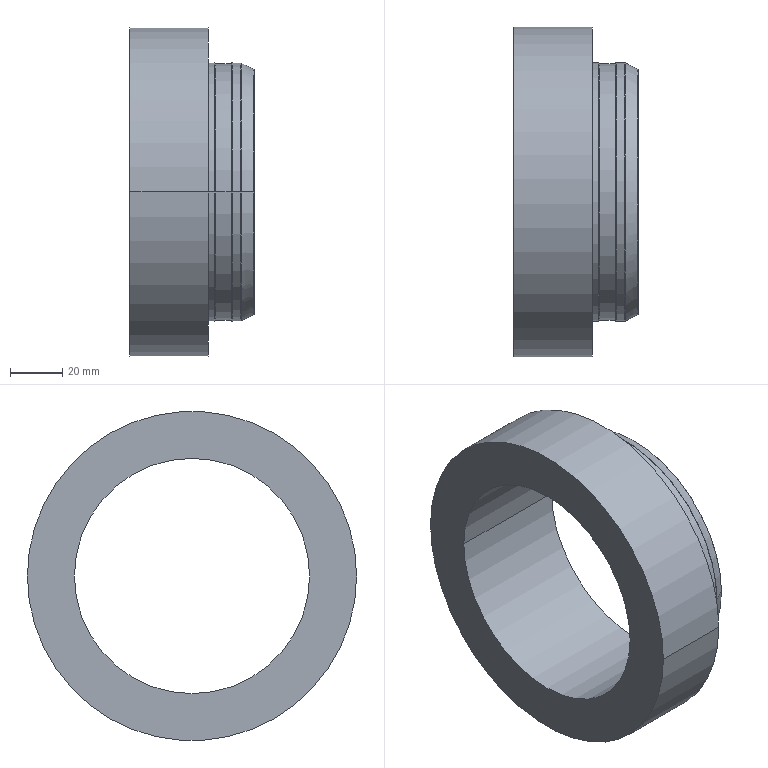Part | SolidWorks | features Revolution 1 | 1 solid | 29 faces | box 47.5 x 126 x 126 mm | volume 203542 mm3 | torus 14 | cylinder 10 | plane 5 | commonest cylinder face diameters 99 x4 90 x2 98 x2 126 x2
STEP:
#1=CARTESIAN_POINT('',(174.371,-47.05,0.));
#2=VERTEX_POINT('',#1);
#3=CARTESIAN_POINT('',(174.371,47.05,0.));
#4=VERTEX_POINT('',#3);
#5=CARTESIAN_POINT('',(174.371,0.,0.));
#6=DIRECTION('',(1.,0.,0.));
#7=DIRECTION('',(0.,1.,0.));
#8=AXIS2_PLACEMENT_3D('',#5,#6,#7);
#9=CIRCLE('',#8,47.05);
#10=EDGE_CURVE('',#2,#4,#9,.T.);
#11=ORIENTED_EDGE('',*,*,#10,.F.);
#12=CARTESIAN_POINT('',(169.544,-49.471,0.));
#13=VERTEX_POINT('',#12);
#14=CARTESIAN_POINT('',(186.323,-76.904,0.));
#15=DIRECTION('',(0.,0.,1.));
#16=DIRECTION('',(0.,-1.,0.));
#17=AXIS2_PLACEMENT_3D('',#14,#15,#16);
#18=CIRCLE('',#17,32.158);
#19=EDGE_CURVE('',#2,#13,#18,.T.);
#20=ORIENTED_EDGE('',*,*,#19,.T.);
#21=CARTESIAN_POINT('',(169.544,49.471,0.));
#22=VERTEX_POINT('',#21);
#23=CARTESIAN_POINT('',(169.544,0.,0.));
#24=DIRECTION('',(1.,0.,0.));
#25=DIRECTION('',(0.,1.,0.));
#26=AXIS2_PLACEMENT_3D('',#23,#24,#25);
#27=CIRCLE('',#26,49.471);
#28=EDGE_CURVE('',#13,#22,#27,.T.);
#29=ORIENTED_EDGE('',*,*,#28,.T.);
#30=CARTESIAN_POINT('',(186.323,76.904,0.));
#31=DIRECTION('',(0.,0.,-1.));
#32=DIRECTION('',(-1.,0.,0.));
#33=AXIS2_PLACEMENT_3D('',#30,#31,#32);
#34=CIRCLE('',#33,32.158);
#35=EDGE_CURVE('',#4,#22,#34,.T.);
#36=ORIENTED_EDGE('',*,*,#35,.F.);
#37=EDGE_LOOP('',(#11,#20,#29,#36));
#38=FACE_OUTER_BOUND('',#37,.T.);
#39=CARTESIAN_POINT('',(186.323,0.,0.));
#40=DIRECTION('',(1.,0.,0.));
#41=DIRECTION('',(0.,1.,0.));
#42=AXIS2_PLACEMENT_3D('',#39,#40,#41);
#43=TOROIDAL_SURFACE('',#42,76.904,32.158);
#44=ADVANCED_FACE('',(#38),#43,.F.);
#45=CARTESIAN_POINT('',(174.371,0.,0.));
#46=DIRECTION('',(1.,0.,0.));
#47=DIRECTION('',(0.,1.,0.));
#48=AXIS2_PLACEMENT_3D('',#45,#46,#47);
#49=CIRCLE('',#48,47.05);
#50=EDGE_CURVE('',#4,#2,#49,.T.);
#51=ORIENTED_EDGE('',*,*,#50,.T.);
#52=CARTESIAN_POINT('',(174.496,-46.864,0.));
#53=VERTEX_POINT('',#52);
#54=CARTESIAN_POINT('',(174.296,-46.864,0.));
#55=DIRECTION('',(0.,0.,1.));
#56=DIRECTION('',(0.,-1.,0.));
#57=AXIS2_PLACEMENT_3D('',#54,#55,#56);
#58=CIRCLE('',#57,0.2);
#59=EDGE_CURVE('',#2,#53,#58,.T.);
#60=ORIENTED_EDGE('',*,*,#59,.T.);
#61=CARTESIAN_POINT('',(174.496,46.864,0.));
#62=VERTEX_POINT('',#61);
#63=CARTESIAN_POINT('',(174.496,0.,0.));
#64=DIRECTION('',(1.,0.,0.));
#65=DIRECTION('',(0.,1.,0.));
#66=AXIS2_PLACEMENT_3D('',#63,#64,#65);
#67=CIRCLE('',#66,46.864);
#68=EDGE_CURVE('',#62,#53,#67,.T.);
#69=ORIENTED_EDGE('',*,*,#68,.F.);
#70=CARTESIAN_POINT('',(174.296,46.864,0.));
#71=DIRECTION('',(0.,0.,-1.));
#72=DIRECTION('',(-1.,0.,0.));
#73=AXIS2_PLACEMENT_3D('',#70,#71,#72);
#74=CIRCLE('',#73,0.2);
#75=EDGE_CURVE('',#4,#62,#74,.T.);
#76=ORIENTED_EDGE('',*,*,#75,.F.);
#77=EDGE_LOOP('',(#51,#60,#69,#76));
#78=FACE_OUTER_BOUND('',#77,.T.);
#79=CARTESIAN_POINT('',(174.296,0.,0.));
#80=DIRECTION('',(1.,0.,0.));
#81=DIRECTION('',(0.,1.,0.));
#82=AXIS2_PLACEMENT_3D('',#79,#80,#81);
#83=TOROIDAL_SURFACE('',#82,46.864,0.2);
#84=ADVANCED_FACE('',(#78),#83,.T.);
#85=CARTESIAN_POINT('',(126.996,-45.,0.));
#86=VERTEX_POINT('',#85);
#87=CARTESIAN_POINT('',(126.996,45.,0.));
#88=VERTEX_POINT('',#87);
#89=CARTESIAN_POINT('',(126.996,0.,0.));
#90=DIRECTION('',(1.,0.,0.));
#91=DIRECTION('',(0.,1.,0.));
#92=AXIS2_PLACEMENT_3D('',#89,#90,#91);
#93=CIRCLE('',#92,45.);
#94=EDGE_CURVE('',#86,#88,#93,.T.);
#95=ORIENTED_EDGE('',*,*,#94,.F.);
#96=CARTESIAN_POINT('',(174.496,-45.,0.));
#97=VERTEX_POINT('',#96);
#98=CARTESIAN_POINT('',(362.346,-45.,0.));
#99=DIRECTION('',(1.,0.,0.));
#100=VECTOR('',#99,1000.);
#101=LINE('',#98,#100);
#102=EDGE_CURVE('',#86,#97,#101,.T.);
#103=ORIENTED_EDGE('',*,*,#102,.T.);
#104=CARTESIAN_POINT('',(174.496,45.,0.));
#105=VERTEX_POINT('',#104);
#106=CARTESIAN_POINT('',(174.496,0.,0.));
#107=DIRECTION('',(1.,0.,0.));
#108=DIRECTION('',(0.,1.,0.));
#109=AXIS2_PLACEMENT_3D('',#106,#107,#108);
#110=CIRCLE('',#109,45.);
#111=EDGE_CURVE('',#97,#105,#110,.T.);
#112=ORIENTED_EDGE('',*,*,#111,.T.);
#113=CARTESIAN_POINT('',(362.346,45.,0.));
#114=DIRECTION('',(1.,0.,0.));
#115=VECTOR('',#114,1000.);
#116=LINE('',#113,#115);
#117=EDGE_CURVE('',#88,#105,#116,.T.);
#118=ORIENTED_EDGE('',*,*,#117,.F.);
#119=EDGE_LOOP('',(#95,#103,#112,#118));
#120=FACE_OUTER_BOUND('',#119,.T.);
#121=CARTESIAN_POINT('',(362.346,0.,0.));
#122=DIRECTION('',(1.,0.,0.));
#123=DIRECTION('',(0.,1.,0.));
#124=AXIS2_PLACEMENT_3D('',#121,#122,#123);
#125=CYLINDRICAL_SURFACE('',#124,45.);
#126=ADVANCED_FACE('',(#120),#125,.F.);
#127=CARTESIAN_POINT('',(126.996,63.,0.));
#128=VERTEX_POINT('',#127);
#129=CARTESIAN_POINT('',(126.996,-63.,0.));
#130=VERTEX_POINT('',#129);
#131=CARTESIAN_POINT('',(126.996,0.,0.));
#132=DIRECTION('',(1.,0.,0.));
#133=DIRECTION('',(0.,1.,0.));
#134=AXIS2_PLACEMENT_3D('',#131,#132,#133);
#135=CIRCLE('',#134,63.);
#136=EDGE_CURVE('',#128,#130,#135,.T.);
#137=ORIENTED_EDGE('',*,*,#136,.T.);
#138=CARTESIAN_POINT('',(156.996,-63.,0.));
#139=VERTEX_POINT('',#138);
#140=CARTESIAN_POINT('',(362.346,-63.,0.));
#141=DIRECTION('',(1.,0.,0.));
#142=VECTOR('',#141,1000.);
#143=LINE('',#140,#142);
#144=EDGE_CURVE('',#130,#139,#143,.T.);
#145=ORIENTED_EDGE('',*,*,#144,.T.);
#146=CARTESIAN_POINT('',(156.996,63.,0.));
#147=VERTEX_POINT('',#146);
#148=CARTESIAN_POINT('',(156.996,0.,0.));
#149=DIRECTION('',(1.,0.,0.));
#150=DIRECTION('',(0.,1.,0.));
#151=AXIS2_PLACEMENT_3D('',#148,#149,#150);
#152=CIRCLE('',#151,63.);
#153=EDGE_CURVE('',#147,#139,#152,.T.);
#154=ORIENTED_EDGE('',*,*,#153,.F.);
#155=CARTESIAN_POINT('',(362.346,63.,0.));
#156=DIRECTION('',(1.,0.,0.));
#157=VECTOR('',#156,1000.);
#158=LINE('',#155,#157);
#159=EDGE_CURVE('',#128,#147,#158,.T.);
#160=ORIENTED_EDGE('',*,*,#159,.F.);
#161=EDGE_LOOP('',(#137,#145,#154,#160));
#162=FACE_OUTER_BOUND('',#161,.T.);
#163=CARTESIAN_POINT('',(362.346,0.,0.));
#164=DIRECTION('',(1.,0.,0.));
#165=DIRECTION('',(0.,1.,0.));
#166=AXIS2_PLACEMENT_3D('',#163,#164,#165);
#167=CYLINDRICAL_SURFACE('',#166,63.);
#168=ADVANCED_FACE('',(#162),#167,.T.);
#169=CARTESIAN_POINT('',(156.996,49.5,0.));
#170=VERTEX_POINT('',#169);
#171=CARTESIAN_POINT('',(156.996,-49.5,0.));
#172=VERTEX_POINT('',#171);
#173=CARTESIAN_POINT('',(156.996,0.,0.));
#174=DIRECTION('',(1.,0.,0.));
#175=DIRECTION('',(0.,1.,0.));
#176=AXIS2_PLACEMENT_3D('',#173,#174,#175);
#177=CIRCLE('',#176,49.5);
#178=EDGE_CURVE('',#170,#172,#177,.T.);
#179=ORIENTED_EDGE('',*,*,#178,.T.);
#180=CARTESIAN_POINT('',(159.296,-49.5,0.));
#181=VERTEX_POINT('',#180);
#182=CARTESIAN_POINT('',(362.346,-49.5,0.));
#183=DIRECTION('',(1.,0.,0.));
#184=VECTOR('',#183,1000.);
#185=LINE('',#182,#184);
#186=EDGE_CURVE('',#172,#181,#185,.T.);
#187=ORIENTED_EDGE('',*,*,#186,.T.);
#188=CARTESIAN_POINT('',(159.296,49.5,0.));
#189=VERTEX_POINT('',#188);
#190=CARTESIAN_POINT('',(159.296,0.,0.));
#191=DIRECTION('',(1.,0.,0.));
#192=DIRECTION('',(0.,1.,0.));
#193=AXIS2_PLACEMENT_3D('',#190,#191,#192);
#194=CIRCLE('',#193,49.5);
#195=EDGE_CURVE('',#189,#181,#194,.T.);
#196=ORIENTED_EDGE('',*,*,#195,.F.);
#197=CARTESIAN_POINT('',(362.346,49.5,0.));
#198=DIRECTION('',(1.,0.,0.));
#199=VECTOR('',#198,1000.);
#200=LINE('',#197,#199);
#201=EDGE_CURVE('',#170,#189,#200,.T.);
#202=ORIENTED_EDGE('',*,*,#201,.F.);
#203=EDGE_LOOP('',(#179,#187,#196,#202));
#204=FACE_OUTER_BOUND('',#203,.T.);
#205=CARTESIAN_POINT('',(362.346,0.,0.));
#206=DIRECTION('',(1.,0.,0.));
#207=DIRECTION('',(0.,1.,0.));
#208=AXIS2_PLACEMENT_3D('',#205,#206,#207);
#209=CYLINDRICAL_SURFACE('',#208,49.5);
#210=ADVANCED_FACE('',(#204),#209,.T.);
#211=ORIENTED_EDGE('',*,*,#195,.T.);
#212=CARTESIAN_POINT('',(159.496,-49.3,0.));
#213=VERTEX_POINT('',#212);
#214=CARTESIAN_POINT('',(159.296,-49.3,0.));
#215=DIRECTION('',(0.,0.,1.));
#216=DIRECTION('',(0.,-1.,0.));
#217=AXIS2_PLACEMENT_3D('',#214,#215,#216);
#218=CIRCLE('',#217,0.2);
#219=EDGE_CURVE('',#181,#213,#218,.T.);
#220=ORIENTED_EDGE('',*,*,#219,.T.);
#221=CARTESIAN_POINT('',(159.496,49.3,0.));
#222=VERTEX_POINT('',#221);
#223=CARTESIAN_POINT('',(159.496,0.,0.));
#224=DIRECTION('',(1.,0.,0.));
#225=DIRECTION('',(0.,1.,0.));
#226=AXIS2_PLACEMENT_3D('',#223,#224,#225);
#227=CIRCLE('',#226,49.3);
#228=EDGE_CURVE('',#222,#213,#227,.T.);
#229=ORIENTED_EDGE('',*,*,#228,.F.);
#230=CARTESIAN_POINT('',(159.296,49.3,0.));
#231=DIRECTION('',(0.,0.,-1.));
#232=DIRECTION('',(-1.,0.,0.));
#233=AXIS2_PLACEMENT_3D('',#230,#231,#232);
#234=CIRCLE('',#233,0.2);
#235=EDGE_CURVE('',#189,#222,#234,.T.);
#236=ORIENTED_EDGE('',*,*,#235,.F.);
#237=EDGE_LOOP('',(#211,#220,#229,#236));
#238=FACE_OUTER_BOUND('',#237,.T.);
#239=CARTESIAN_POINT('',(159.296,0.,0.));
#240=DIRECTION('',(1.,0.,0.));
#241=DIRECTION('',(0.,1.,0.));
#242=AXIS2_PLACEMENT_3D('',#239,#240,#241);
#243=TOROIDAL_SURFACE('',#242,49.3,0.2);
#244=ADVANCED_FACE('',(#238),#243,.T.);
#245=CARTESIAN_POINT('',(159.696,-49.,0.));
#246=VERTEX_POINT('',#245);
#247=CARTESIAN_POINT('',(159.696,49.,0.));
#248=VERTEX_POINT('',#247);
#249=CARTESIAN_POINT('',(159.696,0.,0.));
#250=DIRECTION('',(1.,0.,0.));
#251=DIRECTION('',(0.,1.,0.));
#252=AXIS2_PLACEMENT_3D('',#249,#250,#251);
#253=CIRCLE('',#252,49.);
#254=EDGE_CURVE('',#246,#248,#253,.T.);
#255=ORIENTED_EDGE('',*,*,#254,.F.);
#256=CARTESIAN_POINT('',(159.496,-49.2,0.));
#257=VERTEX_POINT('',#256);
#258=CARTESIAN_POINT('',(159.696,-49.2,0.));
#259=DIRECTION('',(0.,0.,1.));
#260=DIRECTION('',(0.,-1.,0.));
#261=AXIS2_PLACEMENT_3D('',#258,#259,#260);
#262=CIRCLE('',#261,0.2);
#263=EDGE_CURVE('',#246,#257,#262,.T.);
#264=ORIENTED_EDGE('',*,*,#263,.T.);
#265=CARTESIAN_POINT('',(159.496,49.2,0.));
#266=VERTEX_POINT('',#265);
#267=CARTESIAN_POINT('',(159.496,0.,0.));
#268=DIRECTION('',(1.,0.,0.));
#269=DIRECTION('',(0.,1.,0.));
#270=AXIS2_PLACEMENT_3D('',#267,#268,#269);
#271=CIRCLE('',#270,49.2);
#272=EDGE_CURVE('',#257,#266,#271,.T.);
#273=ORIENTED_EDGE('',*,*,#272,.T.);
#274=CARTESIAN_POINT('',(159.696,49.2,0.));
#275=DIRECTION('',(0.,0.,-1.));
#276=DIRECTION('',(-1.,0.,0.));
#277=AXIS2_PLACEMENT_3D('',#274,#275,#276);
#278=CIRCLE('',#277,0.2);
#279=EDGE_CURVE('',#248,#266,#278,.T.);
#280=ORIENTED_EDGE('',*,*,#279,.F.);
#281=EDGE_LOOP('',(#255,#264,#273,#280));
#282=FACE_OUTER_BOUND('',#281,.T.);
#283=CARTESIAN_POINT('',(159.696,0.,0.));
#284=DIRECTION('',(1.,0.,0.));
#285=DIRECTION('',(0.,1.,0.));
#286=AXIS2_PLACEMENT_3D('',#283,#284,#285);
#287=TOROIDAL_SURFACE('',#286,49.2,0.2);
#288=ADVANCED_FACE('',(#282),#287,.F.);
#289=CARTESIAN_POINT('',(159.696,0.,0.));
#290=DIRECTION('',(1.,0.,0.));
#291=DIRECTION('',(0.,1.,0.));
#292=AXIS2_PLACEMENT_3D('',#289,#290,#291);
#293=CIRCLE('',#292,49.);
#294=EDGE_CURVE('',#248,#246,#293,.T.);
#295=ORIENTED_EDGE('',*,*,#294,.T.);
#296=CARTESIAN_POINT('',(165.796,-49.,0.));
#297=VERTEX_POINT('',#296);
#298=CARTESIAN_POINT('',(362.346,-49.,0.));
#299=DIRECTION('',(1.,0.,0.));
#300=VECTOR('',#299,1000.);
#301=LINE('',#298,#300);
#302=EDGE_CURVE('',#246,#297,#301,.T.);
#303=ORIENTED_EDGE('',*,*,#302,.T.);
#304=CARTESIAN_POINT('',(165.796,49.,0.));
#305=VERTEX_POINT('',#304);
#306=CARTESIAN_POINT('',(165.796,0.,0.));
#307=DIRECTION('',(1.,0.,0.));
#308=DIRECTION('',(0.,1.,0.));
#309=AXIS2_PLACEMENT_3D('',#306,#307,#308);
#310=CIRCLE('',#309,49.);
#311=EDGE_CURVE('',#305,#297,#310,.T.);
#312=ORIENTED_EDGE('',*,*,#311,.F.);
#313=CARTESIAN_POINT('',(362.346,49.,0.));
#314=DIRECTION('',(1.,0.,0.));
#315=VECTOR('',#314,1000.);
#316=LINE('',#313,#315);
#317=EDGE_CURVE('',#248,#305,#316,.T.);
#318=ORIENTED_EDGE('',*,*,#317,.F.);
#319=EDGE_LOOP('',(#295,#303,#312,#318));
#320=FACE_OUTER_BOUND('',#319,.T.);
#321=CARTESIAN_POINT('',(362.346,0.,0.));
#322=DIRECTION('',(1.,0.,0.));
#323=DIRECTION('',(0.,1.,0.));
#324=AXIS2_PLACEMENT_3D('',#321,#322,#323);
#325=CYLINDRICAL_SURFACE('',#324,49.);
#326=ADVANCED_FACE('',(#320),#325,.T.);
#327=CARTESIAN_POINT('',(165.996,-49.2,0.));
#328=VERTEX_POINT('',#327);
#329=CARTESIAN_POINT('',(165.996,49.2,0.));
#330=VERTEX_POINT('',#329);
#331=CARTESIAN_POINT('',(165.996,0.,0.));
#332=DIRECTION('',(1.,0.,0.));
#333=DIRECTION('',(0.,1.,0.));
#334=AXIS2_PLACEMENT_3D('',#331,#332,#333);
#335=CIRCLE('',#334,49.2);
#336=EDGE_CURVE('',#328,#330,#335,.T.);
#337=ORIENTED_EDGE('',*,*,#336,.F.);
#338=CARTESIAN_POINT('',(165.796,-49.2,0.));
#339=DIRECTION('',(0.,0.,1.));
#340=DIRECTION('',(0.,-1.,0.));
#341=AXIS2_PLACEMENT_3D('',#338,#339,#340);
#342=CIRCLE('',#341,0.2);
#343=EDGE_CURVE('',#328,#297,#342,.T.);
#344=ORIENTED_EDGE('',*,*,#343,.T.);
#345=CARTESIAN_POINT('',(165.796,0.,0.));
#346=DIRECTION('',(1.,0.,0.));
#347=DIRECTION('',(0.,1.,0.));
#348=AXIS2_PLACEMENT_3D('',#345,#346,#347);
#349=CIRCLE('',#348,49.);
#350=EDGE_CURVE('',#297,#305,#349,.T.);
#351=ORIENTED_EDGE('',*,*,#350,.T.);
#352=CARTESIAN_POINT('',(165.796,49.2,0.));
#353=DIRECTION('',(0.,0.,-1.));
#354=DIRECTION('',(-1.,0.,0.));
#355=AXIS2_PLACEMENT_3D('',#352,#353,#354);
#356=CIRCLE('',#355,0.2);
#357=EDGE_CURVE('',#330,#305,#356,.T.);
#358=ORIENTED_EDGE('',*,*,#357,.F.);
#359=EDGE_LOOP('',(#337,#344,#351,#358));
#360=FACE_OUTER_BOUND('',#359,.T.);
#361=CARTESIAN_POINT('',(165.796,0.,0.));
#362=DIRECTION('',(1.,0.,0.));
#363=DIRECTION('',(0.,1.,0.));
#364=AXIS2_PLACEMENT_3D('',#361,#362,#363);
#365=TOROIDAL_SURFACE('',#364,49.2,0.2);
#366=ADVANCED_FACE('',(#360),#365,.F.);
#367=CARTESIAN_POINT('',(165.996,49.3,0.));
#368=VERTEX_POINT('',#367);
#369=CARTESIAN_POINT('',(165.996,-49.3,0.));
#370=VERTEX_POINT('',#369);
#371=CARTESIAN_POINT('',(165.996,0.,0.));
#372=DIRECTION('',(1.,0.,0.));
#373=DIRECTION('',(0.,1.,0.));
#374=AXIS2_PLACEMENT_3D('',#371,#372,#373);
#375=CIRCLE('',#374,49.3);
#376=EDGE_CURVE('',#368,#370,#375,.T.);
#377=ORIENTED_EDGE('',*,*,#376,.T.);
#378=CARTESIAN_POINT('',(166.196,-49.5,0.));
#379=VERTEX_POINT('',#378);
#380=CARTESIAN_POINT('',(166.196,-49.3,0.));
#381=DIRECTION('',(0.,0.,1.));
#382=DIRECTION('',(0.,-1.,0.));
#383=AXIS2_PLACEMENT_3D('',#380,#381,#382);
#384=CIRCLE('',#383,0.2);
#385=EDGE_CURVE('',#370,#379,#384,.T.);
#386=ORIENTED_EDGE('',*,*,#385,.T.);
#387=CARTESIAN_POINT('',(166.196,49.5,0.));
#388=VERTEX_POINT('',#387);
#389=CARTESIAN_POINT('',(166.196,0.,0.));
#390=DIRECTION('',(1.,0.,0.));
#391=DIRECTION('',(0.,1.,0.));
#392=AXIS2_PLACEMENT_3D('',#389,#390,#391);
#393=CIRCLE('',#392,49.5);
#394=EDGE_CURVE('',#388,#379,#393,.T.);
#395=ORIENTED_EDGE('',*,*,#394,.F.);
#396=CARTESIAN_POINT('',(166.196,49.3,0.));
#397=DIRECTION('',(0.,0.,-1.));
#398=DIRECTION('',(-1.,0.,0.));
#399=AXIS2_PLACEMENT_3D('',#396,#397,#398);
#400=CIRCLE('',#399,0.2);
#401=EDGE_CURVE('',#368,#388,#400,.T.);
#402=ORIENTED_EDGE('',*,*,#401,.F.);
#403=EDGE_LOOP('',(#377,#386,#395,#402));
#404=FACE_OUTER_BOUND('',#403,.T.);
#405=CARTESIAN_POINT('',(166.196,0.,0.));
#406=DIRECTION('',(1.,0.,0.));
#407=DIRECTION('',(0.,1.,0.));
#408=AXIS2_PLACEMENT_3D('',#405,#406,#407);
#409=TOROIDAL_SURFACE('',#408,49.3,0.2);
#410=ADVANCED_FACE('',(#404),#409,.T.);
#411=ORIENTED_EDGE('',*,*,#394,.T.);
#412=CARTESIAN_POINT('',(169.44,-49.5,0.));
#413=VERTEX_POINT('',#412);
#414=CARTESIAN_POINT('',(362.346,-49.5,0.));
#415=DIRECTION('',(1.,0.,0.));
#416=VECTOR('',#415,1000.);
#417=LINE('',#414,#416);
#418=EDGE_CURVE('',#379,#413,#417,.T.);
#419=ORIENTED_EDGE('',*,*,#418,.T.);
#420=CARTESIAN_POINT('',(169.44,49.5,0.));
#421=VERTEX_POINT('',#420);
#422=CARTESIAN_POINT('',(169.44,0.,0.));
#423=DIRECTION('',(1.,0.,0.));
#424=DIRECTION('',(0.,1.,0.));
#425=AXIS2_PLACEMENT_3D('',#422,#423,#424);
#426=CIRCLE('',#425,49.5);
#427=EDGE_CURVE('',#421,#413,#426,.T.);
#428=ORIENTED_EDGE('',*,*,#427,.F.);
#429=CARTESIAN_POINT('',(362.346,49.5,0.));
#430=DIRECTION('',(1.,0.,0.));
#431=VECTOR('',#430,1000.);
#432=LINE('',#429,#431);
#433=EDGE_CURVE('',#388,#421,#432,.T.);
#434=ORIENTED_EDGE('',*,*,#433,.F.);
#435=EDGE_LOOP('',(#411,#419,#428,#434));
#436=FACE_OUTER_BOUND('',#435,.T.);
#437=CARTESIAN_POINT('',(362.346,0.,0.));
#438=DIRECTION('',(1.,0.,0.));
#439=DIRECTION('',(0.,1.,0.));
#440=AXIS2_PLACEMENT_3D('',#437,#438,#439);
#441=CYLINDRICAL_SURFACE('',#440,49.5);
#442=ADVANCED_FACE('',(#436),#441,.T.);
#443=ORIENTED_EDGE('',*,*,#427,.T.);
#444=CARTESIAN_POINT('',(169.44,-49.3,0.));
#445=DIRECTION('',(0.,0.,1.));
#446=DIRECTION('',(0.,-1.,0.));
#447=AXIS2_PLACEMENT_3D('',#444,#445,#446);
#448=CIRCLE('',#447,0.2);
#449=EDGE_CURVE('',#413,#13,#448,.T.);
#450=ORIENTED_EDGE('',*,*,#449,.T.);
#451=CARTESIAN_POINT('',(169.544,0.,0.));
#452=DIRECTION('',(1.,0.,0.));
#453=DIRECTION('',(0.,1.,0.));
#454=AXIS2_PLACEMENT_3D('',#451,#452,#453);
#455=CIRCLE('',#454,49.471);
#456=EDGE_CURVE('',#22,#13,#455,.T.);
#457=ORIENTED_EDGE('',*,*,#456,.F.);
#458=CARTESIAN_POINT('',(169.44,49.3,0.));
#459=DIRECTION('',(0.,0.,-1.));
#460=DIRECTION('',(-1.,0.,0.));
#461=AXIS2_PLACEMENT_3D('',#458,#459,#460);
#462=CIRCLE('',#461,0.2);
#463=EDGE_CURVE('',#421,#22,#462,.T.);
#464=ORIENTED_EDGE('',*,*,#463,.F.);
#465=EDGE_LOOP('',(#443,#450,#457,#464));
#466=FACE_OUTER_BOUND('',#465,.T.);
#467=CARTESIAN_POINT('',(169.44,0.,0.));
#468=DIRECTION('',(1.,0.,0.));
#469=DIRECTION('',(0.,1.,0.));
#470=AXIS2_PLACEMENT_3D('',#467,#468,#469);
#471=TOROIDAL_SURFACE('',#470,49.3,0.2);
#472=ADVANCED_FACE('',(#466),#471,.T.);
#473=ORIENTED_EDGE('',*,*,#449,.F.);
#474=CARTESIAN_POINT('',(169.44,0.,0.));
#475=DIRECTION('',(1.,0.,0.));
#476=DIRECTION('',(0.,1.,0.));
#477=AXIS2_PLACEMENT_3D('',#474,#475,#476);
#478=CIRCLE('',#477,49.5);
#479=EDGE_CURVE('',#413,#421,#478,.T.);
#480=ORIENTED_EDGE('',*,*,#479,.T.);
#481=ORIENTED_EDGE('',*,*,#463,.T.);
#482=ORIENTED_EDGE('',*,*,#28,.F.);
#483=EDGE_LOOP('',(#473,#480,#481,#482));
#484=FACE_OUTER_BOUND('',#483,.T.);
#485=CARTESIAN_POINT('',(169.44,0.,0.));
#486=DIRECTION('',(1.,0.,0.));
#487=DIRECTION('',(0.,1.,0.));
#488=AXIS2_PLACEMENT_3D('',#485,#486,#487);
#489=TOROIDAL_SURFACE('',#488,49.3,0.2);
#490=ADVANCED_FACE('',(#484),#489,.T.);
#491=ORIENTED_EDGE('',*,*,#418,.F.);
#492=CARTESIAN_POINT('',(166.196,0.,0.));
#493=DIRECTION('',(1.,0.,0.));
#494=DIRECTION('',(0.,1.,0.));
#495=AXIS2_PLACEMENT_3D('',#492,#493,#494);
#496=CIRCLE('',#495,49.5);
#497=EDGE_CURVE('',#379,#388,#496,.T.);
#498=ORIENTED_EDGE('',*,*,#497,.T.);
#499=ORIENTED_EDGE('',*,*,#433,.T.);
#500=ORIENTED_EDGE('',*,*,#479,.F.);
#501=EDGE_LOOP('',(#491,#498,#499,#500));
#502=FACE_OUTER_BOUND('',#501,.T.);
#503=CARTESIAN_POINT('',(362.346,0.,0.));
#504=DIRECTION('',(1.,0.,0.));
#505=DIRECTION('',(0.,1.,0.));
#506=AXIS2_PLACEMENT_3D('',#503,#504,#505);
#507=CYLINDRICAL_SURFACE('',#506,49.5);
#508=ADVANCED_FACE('',(#502),#507,.T.);
#509=ORIENTED_EDGE('',*,*,#385,.F.);
#510=CARTESIAN_POINT('',(165.996,0.,0.));
#511=DIRECTION('',(1.,0.,0.));
#512=DIRECTION('',(0.,1.,0.));
#513=AXIS2_PLACEMENT_3D('',#510,#511,#512);
#514=CIRCLE('',#513,49.3);
#515=EDGE_CURVE('',#370,#368,#514,.T.);
#516=ORIENTED_EDGE('',*,*,#515,.T.);
#517=ORIENTED_EDGE('',*,*,#401,.T.);
#518=ORIENTED_EDGE('',*,*,#497,.F.);
#519=EDGE_LOOP('',(#509,#516,#517,#518));
#520=FACE_OUTER_BOUND('',#519,.T.);
#521=CARTESIAN_POINT('',(166.196,0.,0.));
#522=DIRECTION('',(1.,0.,0.));
#523=DIRECTION('',(0.,1.,0.));
#524=AXIS2_PLACEMENT_3D('',#521,#522,#523);
#525=TOROIDAL_SURFACE('',#524,49.3,0.2);
#526=ADVANCED_FACE('',(#520),#525,.T.);
#527=CARTESIAN_POINT('',(165.996,0.,0.));
#528=DIRECTION('',(1.,0.,0.));
#529=DIRECTION('',(0.,1.,0.));
#530=AXIS2_PLACEMENT_3D('',#527,#528,#529);
#531=CIRCLE('',#530,49.2);
#532=EDGE_CURVE('',#330,#328,#531,.T.);
#533=ORIENTED_EDGE('',*,*,#532,.T.);
#534=ORIENTED_EDGE('',*,*,#336,.T.);
#535=EDGE_LOOP('',(#533,#534));
#536=FACE_BOUND('',#535,.T.);
#537=ORIENTED_EDGE('',*,*,#376,.F.);
#538=ORIENTED_EDGE('',*,*,#515,.F.);
#539=EDGE_LOOP('',(#537,#538));
#540=FACE_OUTER_BOUND('',#539,.T.);
#541=CARTESIAN_POINT('',(165.996,49.3,0.));
#542=DIRECTION('',(-1.,0.,0.));
#543=DIRECTION('',(0.,-1.,0.));
#544=AXIS2_PLACEMENT_3D('',#541,#542,#543);
#545=PLANE('',#544);
#546=ADVANCED_FACE('',(#536,#540),#545,.T.);
#547=ORIENTED_EDGE('',*,*,#343,.F.);
#548=ORIENTED_EDGE('',*,*,#532,.F.);
#549=ORIENTED_EDGE('',*,*,#357,.T.);
#550=ORIENTED_EDGE('',*,*,#311,.T.);
#551=EDGE_LOOP('',(#547,#548,#549,#550));
#552=FACE_OUTER_BOUND('',#551,.T.);
#553=CARTESIAN_POINT('',(165.796,0.,0.));
#554=DIRECTION('',(1.,0.,0.));
#555=DIRECTION('',(0.,1.,0.));
#556=AXIS2_PLACEMENT_3D('',#553,#554,#555);
#557=TOROIDAL_SURFACE('',#556,49.2,0.2);
#558=ADVANCED_FACE('',(#552),#557,.F.);
#559=ORIENTED_EDGE('',*,*,#302,.F.);
#560=ORIENTED_EDGE('',*,*,#254,.T.);
#561=ORIENTED_EDGE('',*,*,#317,.T.);
#562=ORIENTED_EDGE('',*,*,#350,.F.);
#563=EDGE_LOOP('',(#559,#560,#561,#562));
#564=FACE_OUTER_BOUND('',#563,.T.);
#565=CARTESIAN_POINT('',(362.346,0.,0.));
#566=DIRECTION('',(1.,0.,0.));
#567=DIRECTION('',(0.,1.,0.));
#568=AXIS2_PLACEMENT_3D('',#565,#566,#567);
#569=CYLINDRICAL_SURFACE('',#568,49.);
#570=ADVANCED_FACE('',(#564),#569,.T.);
#571=ORIENTED_EDGE('',*,*,#263,.F.);
#572=ORIENTED_EDGE('',*,*,#294,.F.);
#573=ORIENTED_EDGE('',*,*,#279,.T.);
#574=CARTESIAN_POINT('',(159.496,0.,0.));
#575=DIRECTION('',(1.,0.,0.));
#576=DIRECTION('',(0.,1.,0.));
#577=AXIS2_PLACEMENT_3D('',#574,#575,#576);
#578=CIRCLE('',#577,49.2);
#579=EDGE_CURVE('',#266,#257,#578,.T.);
#580=ORIENTED_EDGE('',*,*,#579,.T.);
#581=EDGE_LOOP('',(#571,#572,#573,#580));
#582=FACE_OUTER_BOUND('',#581,.T.);
#583=CARTESIAN_POINT('',(159.696,0.,0.));
#584=DIRECTION('',(1.,0.,0.));
#585=DIRECTION('',(0.,1.,0.));
#586=AXIS2_PLACEMENT_3D('',#583,#584,#585);
#587=TOROIDAL_SURFACE('',#586,49.2,0.2);
#588=ADVANCED_FACE('',(#582),#587,.F.);
#589=ORIENTED_EDGE('',*,*,#228,.T.);
#590=CARTESIAN_POINT('',(159.496,0.,0.));
#591=DIRECTION('',(1.,0.,0.));
#592=DIRECTION('',(0.,1.,0.));
#593=AXIS2_PLACEMENT_3D('',#590,#591,#592);
#594=CIRCLE('',#593,49.3);
#595=EDGE_CURVE('',#213,#222,#594,.T.);
#596=ORIENTED_EDGE('',*,*,#595,.T.);
#597=EDGE_LOOP('',(#589,#596));
#598=FACE_OUTER_BOUND('',#597,.T.);
#599=ORIENTED_EDGE('',*,*,#579,.F.);
#600=ORIENTED_EDGE('',*,*,#272,.F.);
#601=EDGE_LOOP('',(#599,#600));
#602=FACE_BOUND('',#601,.T.);
#603=CARTESIAN_POINT('',(159.496,49.3,0.));
#604=DIRECTION('',(1.,0.,0.));
#605=DIRECTION('',(0.,1.,0.));
#606=AXIS2_PLACEMENT_3D('',#603,#604,#605);
#607=PLANE('',#606);
#608=ADVANCED_FACE('',(#598,#602),#607,.T.);
#609=ORIENTED_EDGE('',*,*,#219,.F.);
#610=CARTESIAN_POINT('',(159.296,0.,0.));
#611=DIRECTION('',(1.,0.,0.));
#612=DIRECTION('',(0.,1.,0.));
#613=AXIS2_PLACEMENT_3D('',#610,#611,#612);
#614=CIRCLE('',#613,49.5);
#615=EDGE_CURVE('',#181,#189,#614,.T.);
#616=ORIENTED_EDGE('',*,*,#615,.T.);
#617=ORIENTED_EDGE('',*,*,#235,.T.);
#618=ORIENTED_EDGE('',*,*,#595,.F.);
#619=EDGE_LOOP('',(#609,#616,#617,#618));
#620=FACE_OUTER_BOUND('',#619,.T.);
#621=CARTESIAN_POINT('',(159.296,0.,0.));
#622=DIRECTION('',(1.,0.,0.));
#623=DIRECTION('',(0.,1.,0.));
#624=AXIS2_PLACEMENT_3D('',#621,#622,#623);
#625=TOROIDAL_SURFACE('',#624,49.3,0.2);
#626=ADVANCED_FACE('',(#620),#625,.T.);
#627=ORIENTED_EDGE('',*,*,#186,.F.);
#628=CARTESIAN_POINT('',(156.996,0.,0.));
#629=DIRECTION('',(1.,0.,0.));
#630=DIRECTION('',(0.,1.,0.));
#631=AXIS2_PLACEMENT_3D('',#628,#629,#630);
#632=CIRCLE('',#631,49.5);
#633=EDGE_CURVE('',#172,#170,#632,.T.);
#634=ORIENTED_EDGE('',*,*,#633,.T.);
#635=ORIENTED_EDGE('',*,*,#201,.T.);
#636=ORIENTED_EDGE('',*,*,#615,.F.);
#637=EDGE_LOOP('',(#627,#634,#635,#636));
#638=FACE_OUTER_BOUND('',#637,.T.);
#639=CARTESIAN_POINT('',(362.346,0.,0.));
#640=DIRECTION('',(1.,0.,0.));
#641=DIRECTION('',(0.,1.,0.));
#642=AXIS2_PLACEMENT_3D('',#639,#640,#641);
#643=CYLINDRICAL_SURFACE('',#642,49.5);
#644=ADVANCED_FACE('',(#638),#643,.T.);
#645=ORIENTED_EDGE('',*,*,#153,.T.);
#646=CARTESIAN_POINT('',(156.996,0.,0.));
#647=DIRECTION('',(1.,0.,0.));
#648=DIRECTION('',(0.,1.,0.));
#649=AXIS2_PLACEMENT_3D('',#646,#647,#648);
#650=CIRCLE('',#649,63.);
#651=EDGE_CURVE('',#139,#147,#650,.T.);
#652=ORIENTED_EDGE('',*,*,#651,.T.);
#653=EDGE_LOOP('',(#645,#652));
#654=FACE_OUTER_BOUND('',#653,.T.);
#655=ORIENTED_EDGE('',*,*,#178,.F.);
#656=ORIENTED_EDGE('',*,*,#633,.F.);
#657=EDGE_LOOP('',(#655,#656));
#658=FACE_BOUND('',#657,.T.);
#659=CARTESIAN_POINT('',(156.996,63.,0.));
#660=DIRECTION('',(1.,0.,0.));
#661=DIRECTION('',(0.,1.,0.));
#662=AXIS2_PLACEMENT_3D('',#659,#660,#661);
#663=PLANE('',#662);
#664=ADVANCED_FACE('',(#654,#658),#663,.T.);
#665=ORIENTED_EDGE('',*,*,#144,.F.);
#666=CARTESIAN_POINT('',(126.996,0.,0.));
#667=DIRECTION('',(1.,0.,0.));
#668=DIRECTION('',(0.,1.,0.));
#669=AXIS2_PLACEMENT_3D('',#666,#667,#668);
#670=CIRCLE('',#669,63.);
#671=EDGE_CURVE('',#130,#128,#670,.T.);
#672=ORIENTED_EDGE('',*,*,#671,.T.);
#673=ORIENTED_EDGE('',*,*,#159,.T.);
#674=ORIENTED_EDGE('',*,*,#651,.F.);
#675=EDGE_LOOP('',(#665,#672,#673,#674));
#676=FACE_OUTER_BOUND('',#675,.T.);
#677=CARTESIAN_POINT('',(362.346,0.,0.));
#678=DIRECTION('',(1.,0.,0.));
#679=DIRECTION('',(0.,1.,0.));
#680=AXIS2_PLACEMENT_3D('',#677,#678,#679);
#681=CYLINDRICAL_SURFACE('',#680,63.);
#682=ADVANCED_FACE('',(#676),#681,.T.);
#683=CARTESIAN_POINT('',(126.996,0.,0.));
#684=DIRECTION('',(1.,0.,0.));
#685=DIRECTION('',(0.,1.,0.));
#686=AXIS2_PLACEMENT_3D('',#683,#684,#685);
#687=CIRCLE('',#686,45.);
#688=EDGE_CURVE('',#88,#86,#687,.T.);
#689=ORIENTED_EDGE('',*,*,#688,.T.);
#690=ORIENTED_EDGE('',*,*,#94,.T.);
#691=EDGE_LOOP('',(#689,#690));
#692=FACE_BOUND('',#691,.T.);
#693=ORIENTED_EDGE('',*,*,#136,.F.);
#694=ORIENTED_EDGE('',*,*,#671,.F.);
#695=EDGE_LOOP('',(#693,#694));
#696=FACE_OUTER_BOUND('',#695,.T.);
#697=CARTESIAN_POINT('',(126.996,63.,0.));
#698=DIRECTION('',(-1.,0.,0.));
#699=DIRECTION('',(0.,-1.,0.));
#700=AXIS2_PLACEMENT_3D('',#697,#698,#699);
#701=PLANE('',#700);
#702=ADVANCED_FACE('',(#692,#696),#701,.T.);
#703=ORIENTED_EDGE('',*,*,#102,.F.);
#704=ORIENTED_EDGE('',*,*,#688,.F.);
#705=ORIENTED_EDGE('',*,*,#117,.T.);
#706=CARTESIAN_POINT('',(174.496,0.,0.));
#707=DIRECTION('',(1.,0.,0.));
#708=DIRECTION('',(0.,1.,0.));
#709=AXIS2_PLACEMENT_3D('',#706,#707,#708);
#710=CIRCLE('',#709,45.);
#711=EDGE_CURVE('',#105,#97,#710,.T.);
#712=ORIENTED_EDGE('',*,*,#711,.T.);
#713=EDGE_LOOP('',(#703,#704,#705,#712));
#714=FACE_OUTER_BOUND('',#713,.T.);
#715=CARTESIAN_POINT('',(362.346,0.,0.));
#716=DIRECTION('',(1.,0.,0.));
#717=DIRECTION('',(0.,1.,0.));
#718=AXIS2_PLACEMENT_3D('',#715,#716,#717);
#719=CYLINDRICAL_SURFACE('',#718,45.);
#720=ADVANCED_FACE('',(#714),#719,.F.);
#721=ORIENTED_EDGE('',*,*,#68,.T.);
#722=CARTESIAN_POINT('',(174.496,0.,0.));
#723=DIRECTION('',(1.,0.,0.));
#724=DIRECTION('',(0.,1.,0.));
#725=AXIS2_PLACEMENT_3D('',#722,#723,#724);
#726=CIRCLE('',#725,46.864);
#727=EDGE_CURVE('',#53,#62,#726,.T.);
#728=ORIENTED_EDGE('',*,*,#727,.T.);
#729=EDGE_LOOP('',(#721,#728));
#730=FACE_OUTER_BOUND('',#729,.T.);
#731=ORIENTED_EDGE('',*,*,#711,.F.);
#732=ORIENTED_EDGE('',*,*,#111,.F.);
#733=EDGE_LOOP('',(#731,#732));
#734=FACE_BOUND('',#733,.T.);
#735=CARTESIAN_POINT('',(174.496,46.864,0.));
#736=DIRECTION('',(1.,0.,0.));
#737=DIRECTION('',(0.,1.,0.));
#738=AXIS2_PLACEMENT_3D('',#735,#736,#737);
#739=PLANE('',#738);
#740=ADVANCED_FACE('',(#730,#734),#739,.T.);
#741=ORIENTED_EDGE('',*,*,#59,.F.);
#742=ORIENTED_EDGE('',*,*,#10,.T.);
#743=ORIENTED_EDGE('',*,*,#75,.T.);
#744=ORIENTED_EDGE('',*,*,#727,.F.);
#745=EDGE_LOOP('',(#741,#742,#743,#744));
#746=FACE_OUTER_BOUND('',#745,.T.);
#747=CARTESIAN_POINT('',(174.296,0.,0.));
#748=DIRECTION('',(1.,0.,0.));
#749=DIRECTION('',(0.,1.,0.));
#750=AXIS2_PLACEMENT_3D('',#747,#748,#749);
#751=TOROIDAL_SURFACE('',#750,46.864,0.2);
#752=ADVANCED_FACE('',(#746),#751,.T.);
#753=ORIENTED_EDGE('',*,*,#19,.F.);
#754=ORIENTED_EDGE('',*,*,#50,.F.);
#755=ORIENTED_EDGE('',*,*,#35,.T.);
#756=ORIENTED_EDGE('',*,*,#456,.T.);
#757=EDGE_LOOP('',(#753,#754,#755,#756));
#758=FACE_OUTER_BOUND('',#757,.T.);
#759=CARTESIAN_POINT('',(186.323,0.,0.));
#760=DIRECTION('',(1.,0.,0.));
#761=DIRECTION('',(0.,1.,0.));
#762=AXIS2_PLACEMENT_3D('',#759,#760,#761);
#763=TOROIDAL_SURFACE('',#762,76.904,32.158);
#764=ADVANCED_FACE('',(#758),#763,.F.);
#765=CLOSED_SHELL('',(#44,#84,#126,#168,#210,#244,#288,#326,#366,#410,#442,#472,#490,#508,#526,#546,#558,#570,#588,#608,#626,#644,#664,#682,#702,#720,#740,#752,#764));
#766=MANIFOLD_SOLID_BREP('',#765);
#767=CARTESIAN_POINT('',(0.,0.,0.));
#768=DIRECTION('',(0.,0.,1.));
#769=DIRECTION('',(1.,0.,0.));
#770=AXIS2_PLACEMENT_3D('',#767,#768,#769);
#771=(LENGTH_UNIT()NAMED_UNIT(*)SI_UNIT(.MILLI.,.METRE.));
#772=UNCERTAINTY_MEASURE_WITH_UNIT(LENGTH_MEASURE(0.00001),#771,'','');
#773=(NAMED_UNIT(*)PLANE_ANGLE_UNIT()SI_UNIT($,.RADIAN.));
#774=(NAMED_UNIT(*)SI_UNIT($,.STERADIAN.)SOLID_ANGLE_UNIT());
#775=(GEOMETRIC_REPRESENTATION_CONTEXT(3)GLOBAL_UNCERTAINTY_ASSIGNED_CONTEXT((#772))GLOBAL_UNIT_ASSIGNED_CONTEXT((#771,#773,#774))REPRESENTATION_CONTEXT('',''));
#776=ADVANCED_BREP_SHAPE_REPRESENTATION('',(#766,#770),#775);